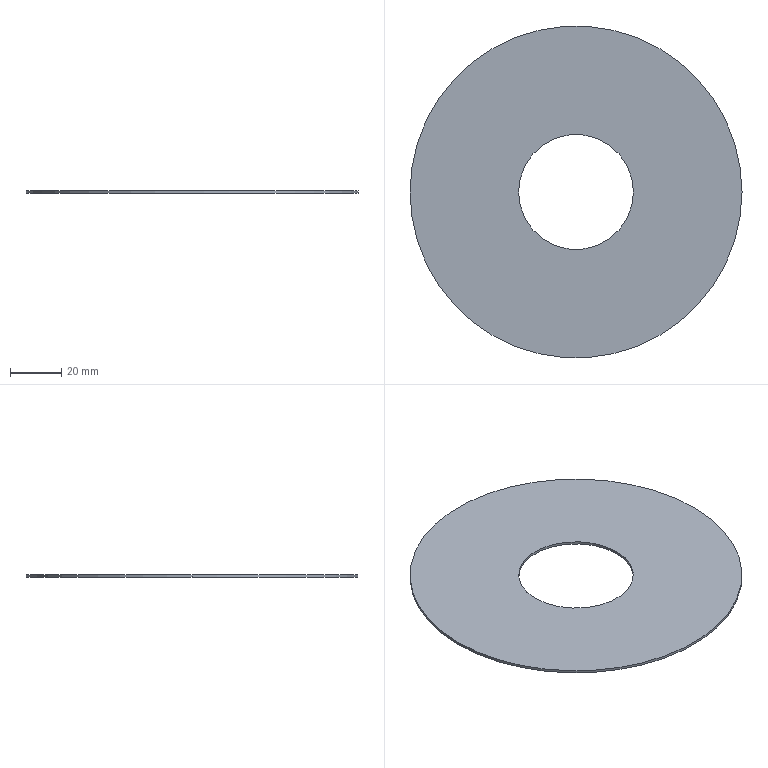Part | SolidWorks | features BaseBody 1 | 1 solid | 6 faces | box 130 x 130 x 1 mm | volume 11683 mm3 | cylinder 4 | plane 2 | commonest cylinder face diameters 45 x2 130 x2
STEP:
#1=CARTESIAN_POINT('',(34.747,463.007,-322.55));
#2=VERTEX_POINT('',#1);
#3=CARTESIAN_POINT('',(79.747,463.007,-322.55));
#4=VERTEX_POINT('',#3);
#5=CARTESIAN_POINT('',(57.247,463.007,-322.55));
#6=DIRECTION('',(0.,0.,1.));
#7=DIRECTION('',(1.,0.,0.));
#8=AXIS2_PLACEMENT_3D('',#5,#6,#7);
#9=CIRCLE('',#8,22.5);
#10=EDGE_CURVE('',#2,#4,#9,.T.);
#11=ORIENTED_EDGE('',*,*,#10,.F.);
#12=CARTESIAN_POINT('',(34.747,463.007,-321.55));
#13=VERTEX_POINT('',#12);
#14=CARTESIAN_POINT('',(34.747,463.007,-322.55));
#15=DIRECTION('',(0.,0.,1.));
#16=VECTOR('',#15,1000.);
#17=LINE('',#14,#16);
#18=EDGE_CURVE('',#2,#13,#17,.T.);
#19=ORIENTED_EDGE('',*,*,#18,.T.);
#20=CARTESIAN_POINT('',(79.747,463.007,-321.55));
#21=VERTEX_POINT('',#20);
#22=CARTESIAN_POINT('',(57.247,463.007,-321.55));
#23=DIRECTION('',(0.,0.,-1.));
#24=DIRECTION('',(1.,0.,0.));
#25=AXIS2_PLACEMENT_3D('',#22,#23,#24);
#26=CIRCLE('',#25,22.5);
#27=EDGE_CURVE('',#21,#13,#26,.T.);
#28=ORIENTED_EDGE('',*,*,#27,.F.);
#29=CARTESIAN_POINT('',(79.747,463.007,-322.55));
#30=DIRECTION('',(0.,0.,1.));
#31=VECTOR('',#30,1000.);
#32=LINE('',#29,#31);
#33=EDGE_CURVE('',#4,#21,#32,.T.);
#34=ORIENTED_EDGE('',*,*,#33,.F.);
#35=EDGE_LOOP('',(#11,#19,#28,#34));
#36=FACE_OUTER_BOUND('',#35,.T.);
#37=CARTESIAN_POINT('',(57.247,463.007,-322.55));
#38=DIRECTION('',(0.,0.,1.));
#39=DIRECTION('',(1.,0.,0.));
#40=AXIS2_PLACEMENT_3D('',#37,#38,#39);
#41=CYLINDRICAL_SURFACE('',#40,22.5);
#42=ADVANCED_FACE('',(#36),#41,.F.);
#43=CARTESIAN_POINT('',(-7.753,463.007,-322.55));
#44=VERTEX_POINT('',#43);
#45=CARTESIAN_POINT('',(122.247,463.007,-322.55));
#46=VERTEX_POINT('',#45);
#47=CARTESIAN_POINT('',(57.247,463.007,-322.55));
#48=DIRECTION('',(0.,0.,-1.));
#49=DIRECTION('',(1.,0.,0.));
#50=AXIS2_PLACEMENT_3D('',#47,#48,#49);
#51=CIRCLE('',#50,65.);
#52=EDGE_CURVE('',#44,#46,#51,.T.);
#53=ORIENTED_EDGE('',*,*,#52,.F.);
#54=CARTESIAN_POINT('',(-7.753,463.007,-321.55));
#55=VERTEX_POINT('',#54);
#56=CARTESIAN_POINT('',(-7.753,463.007,-322.55));
#57=DIRECTION('',(0.,0.,1.));
#58=VECTOR('',#57,1000.);
#59=LINE('',#56,#58);
#60=EDGE_CURVE('',#44,#55,#59,.T.);
#61=ORIENTED_EDGE('',*,*,#60,.T.);
#62=CARTESIAN_POINT('',(122.247,463.007,-321.55));
#63=VERTEX_POINT('',#62);
#64=CARTESIAN_POINT('',(57.247,463.007,-321.55));
#65=DIRECTION('',(0.,0.,-1.));
#66=DIRECTION('',(1.,0.,0.));
#67=AXIS2_PLACEMENT_3D('',#64,#65,#66);
#68=CIRCLE('',#67,65.);
#69=EDGE_CURVE('',#55,#63,#68,.T.);
#70=ORIENTED_EDGE('',*,*,#69,.T.);
#71=CARTESIAN_POINT('',(122.247,463.007,-322.55));
#72=DIRECTION('',(0.,0.,1.));
#73=VECTOR('',#72,1000.);
#74=LINE('',#71,#73);
#75=EDGE_CURVE('',#46,#63,#74,.T.);
#76=ORIENTED_EDGE('',*,*,#75,.F.);
#77=EDGE_LOOP('',(#53,#61,#70,#76));
#78=FACE_OUTER_BOUND('',#77,.T.);
#79=CARTESIAN_POINT('',(57.247,463.007,-322.55));
#80=DIRECTION('',(0.,0.,1.));
#81=DIRECTION('',(1.,0.,0.));
#82=AXIS2_PLACEMENT_3D('',#79,#80,#81);
#83=CYLINDRICAL_SURFACE('',#82,65.);
#84=ADVANCED_FACE('',(#78),#83,.T.);
#85=CARTESIAN_POINT('',(57.247,463.007,-322.55));
#86=DIRECTION('',(0.,0.,1.));
#87=DIRECTION('',(1.,0.,0.));
#88=AXIS2_PLACEMENT_3D('',#85,#86,#87);
#89=CIRCLE('',#88,22.5);
#90=EDGE_CURVE('',#4,#2,#89,.T.);
#91=ORIENTED_EDGE('',*,*,#90,.T.);
#92=ORIENTED_EDGE('',*,*,#10,.T.);
#93=EDGE_LOOP('',(#91,#92));
#94=FACE_BOUND('',#93,.T.);
#95=CARTESIAN_POINT('',(57.247,463.007,-322.55));
#96=DIRECTION('',(0.,0.,-1.));
#97=DIRECTION('',(1.,0.,0.));
#98=AXIS2_PLACEMENT_3D('',#95,#96,#97);
#99=CIRCLE('',#98,65.);
#100=EDGE_CURVE('',#46,#44,#99,.T.);
#101=ORIENTED_EDGE('',*,*,#100,.T.);
#102=ORIENTED_EDGE('',*,*,#52,.T.);
#103=EDGE_LOOP('',(#101,#102));
#104=FACE_OUTER_BOUND('',#103,.T.);
#105=CARTESIAN_POINT('',(57.247,463.007,-322.55));
#106=DIRECTION('',(0.,0.,-1.));
#107=DIRECTION('',(-1.,0.,0.));
#108=AXIS2_PLACEMENT_3D('',#105,#106,#107);
#109=PLANE('',#108);
#110=ADVANCED_FACE('',(#94,#104),#109,.T.);
#111=ORIENTED_EDGE('',*,*,#18,.F.);
#112=ORIENTED_EDGE('',*,*,#90,.F.);
#113=ORIENTED_EDGE('',*,*,#33,.T.);
#114=CARTESIAN_POINT('',(57.247,463.007,-321.55));
#115=DIRECTION('',(0.,0.,-1.));
#116=DIRECTION('',(1.,0.,0.));
#117=AXIS2_PLACEMENT_3D('',#114,#115,#116);
#118=CIRCLE('',#117,22.5);
#119=EDGE_CURVE('',#13,#21,#118,.T.);
#120=ORIENTED_EDGE('',*,*,#119,.F.);
#121=EDGE_LOOP('',(#111,#112,#113,#120));
#122=FACE_OUTER_BOUND('',#121,.T.);
#123=CARTESIAN_POINT('',(57.247,463.007,-322.55));
#124=DIRECTION('',(0.,0.,1.));
#125=DIRECTION('',(1.,0.,0.));
#126=AXIS2_PLACEMENT_3D('',#123,#124,#125);
#127=CYLINDRICAL_SURFACE('',#126,22.5);
#128=ADVANCED_FACE('',(#122),#127,.F.);
#129=ORIENTED_EDGE('',*,*,#60,.F.);
#130=ORIENTED_EDGE('',*,*,#100,.F.);
#131=ORIENTED_EDGE('',*,*,#75,.T.);
#132=CARTESIAN_POINT('',(57.247,463.007,-321.55));
#133=DIRECTION('',(0.,0.,-1.));
#134=DIRECTION('',(1.,0.,0.));
#135=AXIS2_PLACEMENT_3D('',#132,#133,#134);
#136=CIRCLE('',#135,65.);
#137=EDGE_CURVE('',#63,#55,#136,.T.);
#138=ORIENTED_EDGE('',*,*,#137,.T.);
#139=EDGE_LOOP('',(#129,#130,#131,#138));
#140=FACE_OUTER_BOUND('',#139,.T.);
#141=CARTESIAN_POINT('',(57.247,463.007,-322.55));
#142=DIRECTION('',(0.,0.,1.));
#143=DIRECTION('',(1.,0.,0.));
#144=AXIS2_PLACEMENT_3D('',#141,#142,#143);
#145=CYLINDRICAL_SURFACE('',#144,65.);
#146=ADVANCED_FACE('',(#140),#145,.T.);
#147=ORIENTED_EDGE('',*,*,#27,.T.);
#148=ORIENTED_EDGE('',*,*,#119,.T.);
#149=EDGE_LOOP('',(#147,#148));
#150=FACE_BOUND('',#149,.T.);
#151=ORIENTED_EDGE('',*,*,#137,.F.);
#152=ORIENTED_EDGE('',*,*,#69,.F.);
#153=EDGE_LOOP('',(#151,#152));
#154=FACE_OUTER_BOUND('',#153,.T.);
#155=CARTESIAN_POINT('',(57.247,463.007,-321.55));
#156=DIRECTION('',(0.,0.,-1.));
#157=DIRECTION('',(-1.,0.,0.));
#158=AXIS2_PLACEMENT_3D('',#155,#156,#157);
#159=PLANE('',#158);
#160=ADVANCED_FACE('',(#150,#154),#159,.F.);
#161=CLOSED_SHELL('',(#42,#84,#110,#128,#146,#160));
#162=MANIFOLD_SOLID_BREP('',#161);
#163=CARTESIAN_POINT('',(0.,0.,0.));
#164=DIRECTION('',(0.,0.,1.));
#165=DIRECTION('',(1.,0.,0.));
#166=AXIS2_PLACEMENT_3D('',#163,#164,#165);
#167=(LENGTH_UNIT()NAMED_UNIT(*)SI_UNIT(.MILLI.,.METRE.));
#168=UNCERTAINTY_MEASURE_WITH_UNIT(LENGTH_MEASURE(0.00001),#167,'','');
#169=(NAMED_UNIT(*)PLANE_ANGLE_UNIT()SI_UNIT($,.RADIAN.));
#170=(NAMED_UNIT(*)SI_UNIT($,.STERADIAN.)SOLID_ANGLE_UNIT());
#171=(GEOMETRIC_REPRESENTATION_CONTEXT(3)GLOBAL_UNCERTAINTY_ASSIGNED_CONTEXT((#168))GLOBAL_UNIT_ASSIGNED_CONTEXT((#167,#169,#170))REPRESENTATION_CONTEXT('',''));
#172=ADVANCED_BREP_SHAPE_REPRESENTATION('',(#162,#166),#171);